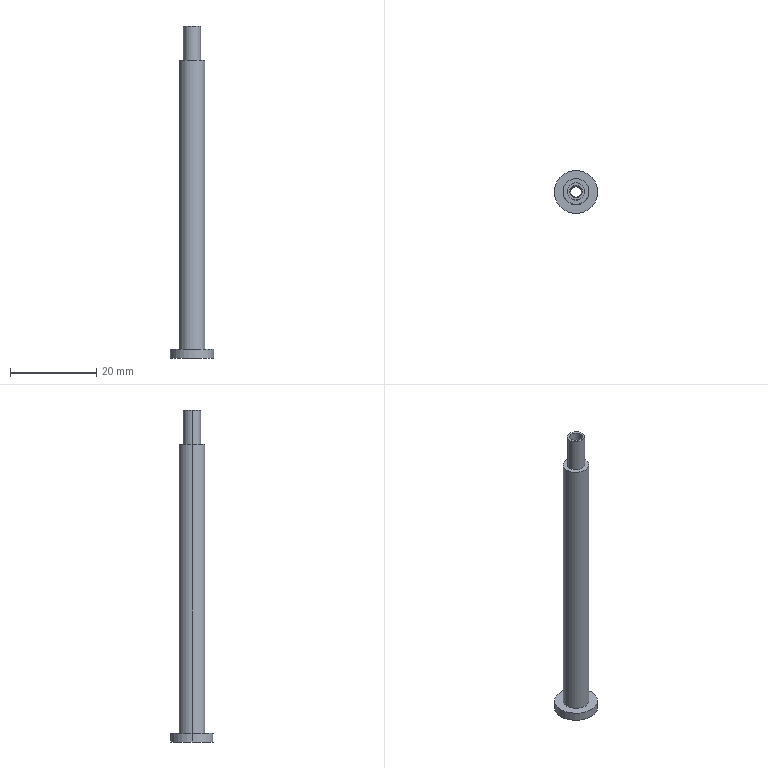Part | SolidWorks | features BaseBody 1 | 1 solid | 16 faces | box 10 x 10 x 77 mm | volume 1624 mm3 | cylinder 10 | plane 4 | cone 2 | commonest cylinder face diameters 2.459 x2 3 x2 4 x2 6 x2 10 x2
STEP:
#1=CARTESIAN_POINT('',(3.,0.,2.));
#2=VERTEX_POINT('',#1);
#3=CARTESIAN_POINT('',(-3.,0.,2.));
#4=VERTEX_POINT('',#3);
#5=CARTESIAN_POINT('',(0.,0.,2.));
#6=DIRECTION('',(0.,0.,1.));
#7=DIRECTION('',(1.,0.,0.));
#8=AXIS2_PLACEMENT_3D('',#5,#6,#7);
#9=CIRCLE('',#8,3.);
#10=EDGE_CURVE('',#2,#4,#9,.T.);
#11=ORIENTED_EDGE('',*,*,#10,.T.);
#12=CARTESIAN_POINT('',(-3.,0.,69.));
#13=VERTEX_POINT('',#12);
#14=CARTESIAN_POINT('',(-3.,0.,2.));
#15=DIRECTION('',(0.,0.,1.));
#16=VECTOR('',#15,1000.);
#17=LINE('',#14,#16);
#18=EDGE_CURVE('',#4,#13,#17,.T.);
#19=ORIENTED_EDGE('',*,*,#18,.T.);
#20=CARTESIAN_POINT('',(3.,0.,69.));
#21=VERTEX_POINT('',#20);
#22=CARTESIAN_POINT('',(0.,0.,69.));
#23=DIRECTION('',(0.,0.,-1.));
#24=DIRECTION('',(1.,0.,0.));
#25=AXIS2_PLACEMENT_3D('',#22,#23,#24);
#26=CIRCLE('',#25,3.);
#27=EDGE_CURVE('',#13,#21,#26,.T.);
#28=ORIENTED_EDGE('',*,*,#27,.T.);
#29=CARTESIAN_POINT('',(3.,0.,2.));
#30=DIRECTION('',(0.,0.,1.));
#31=VECTOR('',#30,1000.);
#32=LINE('',#29,#31);
#33=EDGE_CURVE('',#2,#21,#32,.T.);
#34=ORIENTED_EDGE('',*,*,#33,.F.);
#35=EDGE_LOOP('',(#11,#19,#28,#34));
#36=FACE_OUTER_BOUND('',#35,.T.);
#37=CARTESIAN_POINT('',(0.,0.,2.));
#38=DIRECTION('',(0.,0.,1.));
#39=DIRECTION('',(1.,0.,0.));
#40=AXIS2_PLACEMENT_3D('',#37,#38,#39);
#41=CYLINDRICAL_SURFACE('',#40,3.);
#42=ADVANCED_FACE('',(#36),#41,.T.);
#43=CARTESIAN_POINT('',(5.,0.,0.));
#44=VERTEX_POINT('',#43);
#45=CARTESIAN_POINT('',(-5.,0.,0.));
#46=VERTEX_POINT('',#45);
#47=CARTESIAN_POINT('',(0.,0.,0.));
#48=DIRECTION('',(0.,0.,1.));
#49=DIRECTION('',(1.,0.,0.));
#50=AXIS2_PLACEMENT_3D('',#47,#48,#49);
#51=CIRCLE('',#50,5.);
#52=EDGE_CURVE('',#44,#46,#51,.T.);
#53=ORIENTED_EDGE('',*,*,#52,.T.);
#54=CARTESIAN_POINT('',(-5.,0.,2.));
#55=VERTEX_POINT('',#54);
#56=CARTESIAN_POINT('',(-5.,0.,0.));
#57=DIRECTION('',(0.,0.,1.));
#58=VECTOR('',#57,1000.);
#59=LINE('',#56,#58);
#60=EDGE_CURVE('',#46,#55,#59,.T.);
#61=ORIENTED_EDGE('',*,*,#60,.T.);
#62=CARTESIAN_POINT('',(5.,0.,2.));
#63=VERTEX_POINT('',#62);
#64=CARTESIAN_POINT('',(0.,0.,2.));
#65=DIRECTION('',(0.,0.,-1.));
#66=DIRECTION('',(1.,0.,0.));
#67=AXIS2_PLACEMENT_3D('',#64,#65,#66);
#68=CIRCLE('',#67,5.);
#69=EDGE_CURVE('',#55,#63,#68,.T.);
#70=ORIENTED_EDGE('',*,*,#69,.T.);
#71=CARTESIAN_POINT('',(5.,0.,0.));
#72=DIRECTION('',(0.,0.,1.));
#73=VECTOR('',#72,1000.);
#74=LINE('',#71,#73);
#75=EDGE_CURVE('',#44,#63,#74,.T.);
#76=ORIENTED_EDGE('',*,*,#75,.F.);
#77=EDGE_LOOP('',(#53,#61,#70,#76));
#78=FACE_OUTER_BOUND('',#77,.T.);
#79=CARTESIAN_POINT('',(0.,0.,0.));
#80=DIRECTION('',(0.,0.,1.));
#81=DIRECTION('',(1.,0.,0.));
#82=AXIS2_PLACEMENT_3D('',#79,#80,#81);
#83=CYLINDRICAL_SURFACE('',#82,5.);
#84=ADVANCED_FACE('',(#78),#83,.T.);
#85=CARTESIAN_POINT('',(-2.,0.,77.));
#86=VERTEX_POINT('',#85);
#87=CARTESIAN_POINT('',(2.,0.,77.));
#88=VERTEX_POINT('',#87);
#89=CARTESIAN_POINT('',(0.,0.,77.));
#90=DIRECTION('',(0.,0.,-1.));
#91=DIRECTION('',(-1.,0.,0.));
#92=AXIS2_PLACEMENT_3D('',#89,#90,#91);
#93=CIRCLE('',#92,2.);
#94=EDGE_CURVE('',#86,#88,#93,.T.);
#95=ORIENTED_EDGE('',*,*,#94,.T.);
#96=CARTESIAN_POINT('',(2.,0.,69.));
#97=VERTEX_POINT('',#96);
#98=CARTESIAN_POINT('',(2.,0.,77.));
#99=DIRECTION('',(0.,0.,-1.));
#100=VECTOR('',#99,1000.);
#101=LINE('',#98,#100);
#102=EDGE_CURVE('',#88,#97,#101,.T.);
#103=ORIENTED_EDGE('',*,*,#102,.T.);
#104=CARTESIAN_POINT('',(-2.,0.,69.));
#105=VERTEX_POINT('',#104);
#106=CARTESIAN_POINT('',(0.,0.,69.));
#107=DIRECTION('',(0.,0.,1.));
#108=DIRECTION('',(-1.,0.,0.));
#109=AXIS2_PLACEMENT_3D('',#106,#107,#108);
#110=CIRCLE('',#109,2.);
#111=EDGE_CURVE('',#97,#105,#110,.T.);
#112=ORIENTED_EDGE('',*,*,#111,.T.);
#113=CARTESIAN_POINT('',(-2.,0.,77.));
#114=DIRECTION('',(0.,0.,-1.));
#115=VECTOR('',#114,1000.);
#116=LINE('',#113,#115);
#117=EDGE_CURVE('',#86,#105,#116,.T.);
#118=ORIENTED_EDGE('',*,*,#117,.F.);
#119=EDGE_LOOP('',(#95,#103,#112,#118));
#120=FACE_OUTER_BOUND('',#119,.T.);
#121=CARTESIAN_POINT('',(0.,0.,77.));
#122=DIRECTION('',(0.,0.,-1.));
#123=DIRECTION('',(-1.,0.,0.));
#124=AXIS2_PLACEMENT_3D('',#121,#122,#123);
#125=CYLINDRICAL_SURFACE('',#124,2.);
#126=ADVANCED_FACE('',(#120),#125,.T.);
#127=CARTESIAN_POINT('',(1.23,0.,6.837));
#128=VERTEX_POINT('',#127);
#129=CARTESIAN_POINT('',(0.,-1.23,6.837));
#130=VERTEX_POINT('',#129);
#131=CARTESIAN_POINT('',(0.,0.,6.837));
#132=DIRECTION('',(0.,0.,-1.));
#133=DIRECTION('',(-1.,0.,0.));
#134=AXIS2_PLACEMENT_3D('',#131,#132,#133);
#135=CIRCLE('',#134,1.23);
#136=EDGE_CURVE('',#128,#130,#135,.T.);
#137=ORIENTED_EDGE('',*,*,#136,.F.);
#138=CARTESIAN_POINT('',(1.23,0.,0.));
#139=VERTEX_POINT('',#138);
#140=CARTESIAN_POINT('',(1.23,0.,5.));
#141=DIRECTION('',(0.,0.,-1.));
#142=VECTOR('',#141,1000.);
#143=LINE('',#140,#142);
#144=EDGE_CURVE('',#128,#139,#143,.T.);
#145=ORIENTED_EDGE('',*,*,#144,.T.);
#146=CARTESIAN_POINT('',(-1.23,0.,0.));
#147=VERTEX_POINT('',#146);
#148=CARTESIAN_POINT('',(0.,0.,0.));
#149=DIRECTION('',(0.,0.,1.));
#150=DIRECTION('',(-1.,0.,0.));
#151=AXIS2_PLACEMENT_3D('',#148,#149,#150);
#152=CIRCLE('',#151,1.23);
#153=EDGE_CURVE('',#147,#139,#152,.T.);
#154=ORIENTED_EDGE('',*,*,#153,.F.);
#155=CARTESIAN_POINT('',(-1.23,0.,6.837));
#156=VERTEX_POINT('',#155);
#157=CARTESIAN_POINT('',(-1.23,0.,5.));
#158=DIRECTION('',(0.,0.,-1.));
#159=VECTOR('',#158,1000.);
#160=LINE('',#157,#159);
#161=EDGE_CURVE('',#156,#147,#160,.T.);
#162=ORIENTED_EDGE('',*,*,#161,.F.);
#163=CARTESIAN_POINT('',(0.,0.,6.837));
#164=DIRECTION('',(0.,0.,-1.));
#165=DIRECTION('',(-1.,0.,0.));
#166=AXIS2_PLACEMENT_3D('',#163,#164,#165);
#167=CIRCLE('',#166,1.23);
#168=EDGE_CURVE('',#130,#156,#167,.T.);
#169=ORIENTED_EDGE('',*,*,#168,.F.);
#170=EDGE_LOOP('',(#137,#145,#154,#162,#169));
#171=FACE_OUTER_BOUND('',#170,.T.);
#172=CARTESIAN_POINT('',(0.,0.,5.));
#173=DIRECTION('',(0.,0.,-1.));
#174=DIRECTION('',(-1.,0.,0.));
#175=AXIS2_PLACEMENT_3D('',#172,#173,#174);
#176=CYLINDRICAL_SURFACE('',#175,1.23);
#177=ADVANCED_FACE('',(#171),#176,.F.);
#178=CARTESIAN_POINT('',(-1.5,0.,7.));
#179=VERTEX_POINT('',#178);
#180=CARTESIAN_POINT('',(0.,-1.5,7.));
#181=VERTEX_POINT('',#180);
#182=CARTESIAN_POINT('',(0.,0.,7.));
#183=DIRECTION('',(0.,0.,1.));
#184=DIRECTION('',(1.,0.,0.));
#185=AXIS2_PLACEMENT_3D('',#182,#183,#184);
#186=CIRCLE('',#185,1.5);
#187=EDGE_CURVE('',#179,#181,#186,.T.);
#188=ORIENTED_EDGE('',*,*,#187,.F.);
#189=CARTESIAN_POINT('',(-1.5,0.,77.));
#190=VERTEX_POINT('',#189);
#191=CARTESIAN_POINT('',(-1.5,0.,42.));
#192=DIRECTION('',(0.,0.,1.));
#193=VECTOR('',#192,1000.);
#194=LINE('',#191,#193);
#195=EDGE_CURVE('',#179,#190,#194,.T.);
#196=ORIENTED_EDGE('',*,*,#195,.T.);
#197=CARTESIAN_POINT('',(1.5,0.,77.));
#198=VERTEX_POINT('',#197);
#199=CARTESIAN_POINT('',(0.,0.,77.));
#200=DIRECTION('',(0.,0.,1.));
#201=DIRECTION('',(1.,0.,0.));
#202=AXIS2_PLACEMENT_3D('',#199,#200,#201);
#203=CIRCLE('',#202,1.5);
#204=EDGE_CURVE('',#190,#198,#203,.T.);
#205=ORIENTED_EDGE('',*,*,#204,.T.);
#206=CARTESIAN_POINT('',(1.5,0.,7.));
#207=VERTEX_POINT('',#206);
#208=CARTESIAN_POINT('',(1.5,0.,42.));
#209=DIRECTION('',(0.,0.,1.));
#210=VECTOR('',#209,1000.);
#211=LINE('',#208,#210);
#212=EDGE_CURVE('',#207,#198,#211,.T.);
#213=ORIENTED_EDGE('',*,*,#212,.F.);
#214=CARTESIAN_POINT('',(0.,0.,7.));
#215=DIRECTION('',(0.,0.,1.));
#216=DIRECTION('',(1.,0.,0.));
#217=AXIS2_PLACEMENT_3D('',#214,#215,#216);
#218=CIRCLE('',#217,1.5);
#219=EDGE_CURVE('',#181,#207,#218,.T.);
#220=ORIENTED_EDGE('',*,*,#219,.F.);
#221=EDGE_LOOP('',(#188,#196,#205,#213,#220));
#222=FACE_OUTER_BOUND('',#221,.T.);
#223=CARTESIAN_POINT('',(0.,0.,42.));
#224=DIRECTION('',(0.,0.,1.));
#225=DIRECTION('',(1.,0.,0.));
#226=AXIS2_PLACEMENT_3D('',#223,#224,#225);
#227=CYLINDRICAL_SURFACE('',#226,1.5);
#228=ADVANCED_FACE('',(#222),#227,.F.);
#229=ORIENTED_EDGE('',*,*,#168,.T.);
#230=CARTESIAN_POINT('',(0.,1.23,6.837));
#231=VERTEX_POINT('',#230);
#232=CARTESIAN_POINT('',(0.,0.,6.837));
#233=DIRECTION('',(0.,0.,-1.));
#234=DIRECTION('',(-1.,0.,0.));
#235=AXIS2_PLACEMENT_3D('',#232,#233,#234);
#236=CIRCLE('',#235,1.23);
#237=EDGE_CURVE('',#156,#231,#236,.T.);
#238=ORIENTED_EDGE('',*,*,#237,.T.);
#239=CARTESIAN_POINT('',(0.,1.5,7.));
#240=VERTEX_POINT('',#239);
#241=CARTESIAN_POINT('',(0.,1.5,7.));
#242=DIRECTION('',(0.,0.8572,0.515));
#243=VECTOR('',#242,1000.);
#244=LINE('',#241,#243);
#245=EDGE_CURVE('',#231,#240,#244,.T.);
#246=ORIENTED_EDGE('',*,*,#245,.T.);
#247=CARTESIAN_POINT('',(0.,0.,7.));
#248=DIRECTION('',(0.,0.,1.));
#249=DIRECTION('',(1.,0.,0.));
#250=AXIS2_PLACEMENT_3D('',#247,#248,#249);
#251=CIRCLE('',#250,1.5);
#252=EDGE_CURVE('',#240,#179,#251,.T.);
#253=ORIENTED_EDGE('',*,*,#252,.T.);
#254=ORIENTED_EDGE('',*,*,#187,.T.);
#255=CARTESIAN_POINT('',(0.,-1.5,7.));
#256=DIRECTION('',(0.,-0.8572,0.515));
#257=VECTOR('',#256,1000.);
#258=LINE('',#255,#257);
#259=EDGE_CURVE('',#130,#181,#258,.T.);
#260=ORIENTED_EDGE('',*,*,#259,.F.);
#261=EDGE_LOOP('',(#229,#238,#246,#253,#254,#260));
#262=FACE_OUTER_BOUND('',#261,.T.);
#263=CARTESIAN_POINT('',(0.,0.,7.));
#264=DIRECTION('',(0.,0.,1.));
#265=DIRECTION('',(0.,-1.,0.));
#266=AXIS2_PLACEMENT_3D('',#263,#264,#265);
#267=CONICAL_SURFACE('',#266,1.5,1.03);
#268=ADVANCED_FACE('',(#262),#267,.F.);
#269=ORIENTED_EDGE('',*,*,#18,.F.);
#270=CARTESIAN_POINT('',(0.,0.,2.));
#271=DIRECTION('',(0.,0.,1.));
#272=DIRECTION('',(1.,0.,0.));
#273=AXIS2_PLACEMENT_3D('',#270,#271,#272);
#274=CIRCLE('',#273,3.);
#275=EDGE_CURVE('',#4,#2,#274,.T.);
#276=ORIENTED_EDGE('',*,*,#275,.T.);
#277=ORIENTED_EDGE('',*,*,#33,.T.);
#278=CARTESIAN_POINT('',(0.,0.,69.));
#279=DIRECTION('',(0.,0.,-1.));
#280=DIRECTION('',(1.,0.,0.));
#281=AXIS2_PLACEMENT_3D('',#278,#279,#280);
#282=CIRCLE('',#281,3.);
#283=EDGE_CURVE('',#21,#13,#282,.T.);
#284=ORIENTED_EDGE('',*,*,#283,.T.);
#285=EDGE_LOOP('',(#269,#276,#277,#284));
#286=FACE_OUTER_BOUND('',#285,.T.);
#287=CARTESIAN_POINT('',(0.,0.,2.));
#288=DIRECTION('',(0.,0.,1.));
#289=DIRECTION('',(1.,0.,0.));
#290=AXIS2_PLACEMENT_3D('',#287,#288,#289);
#291=CYLINDRICAL_SURFACE('',#290,3.);
#292=ADVANCED_FACE('',(#286),#291,.T.);
#293=ORIENTED_EDGE('',*,*,#10,.F.);
#294=ORIENTED_EDGE('',*,*,#275,.F.);
#295=EDGE_LOOP('',(#293,#294));
#296=FACE_BOUND('',#295,.T.);
#297=CARTESIAN_POINT('',(0.,0.,2.));
#298=DIRECTION('',(0.,0.,-1.));
#299=DIRECTION('',(1.,0.,0.));
#300=AXIS2_PLACEMENT_3D('',#297,#298,#299);
#301=CIRCLE('',#300,5.);
#302=EDGE_CURVE('',#63,#55,#301,.T.);
#303=ORIENTED_EDGE('',*,*,#302,.F.);
#304=ORIENTED_EDGE('',*,*,#69,.F.);
#305=EDGE_LOOP('',(#303,#304));
#306=FACE_OUTER_BOUND('',#305,.T.);
#307=CARTESIAN_POINT('',(0.,0.,2.));
#308=DIRECTION('',(0.,0.,-1.));
#309=DIRECTION('',(-1.,0.,0.));
#310=AXIS2_PLACEMENT_3D('',#307,#308,#309);
#311=PLANE('',#310);
#312=ADVANCED_FACE('',(#296,#306),#311,.F.);
#313=CARTESIAN_POINT('',(0.,0.,69.));
#314=DIRECTION('',(0.,0.,1.));
#315=DIRECTION('',(-1.,0.,0.));
#316=AXIS2_PLACEMENT_3D('',#313,#314,#315);
#317=CIRCLE('',#316,2.);
#318=EDGE_CURVE('',#105,#97,#317,.T.);
#319=ORIENTED_EDGE('',*,*,#318,.F.);
#320=ORIENTED_EDGE('',*,*,#111,.F.);
#321=EDGE_LOOP('',(#319,#320));
#322=FACE_BOUND('',#321,.T.);
#323=ORIENTED_EDGE('',*,*,#283,.F.);
#324=ORIENTED_EDGE('',*,*,#27,.F.);
#325=EDGE_LOOP('',(#323,#324));
#326=FACE_OUTER_BOUND('',#325,.T.);
#327=CARTESIAN_POINT('',(0.,0.,69.));
#328=DIRECTION('',(0.,0.,-1.));
#329=DIRECTION('',(-1.,0.,0.));
#330=AXIS2_PLACEMENT_3D('',#327,#328,#329);
#331=PLANE('',#330);
#332=ADVANCED_FACE('',(#322,#326),#331,.F.);
#333=ORIENTED_EDGE('',*,*,#60,.F.);
#334=CARTESIAN_POINT('',(0.,0.,0.));
#335=DIRECTION('',(0.,0.,1.));
#336=DIRECTION('',(1.,0.,0.));
#337=AXIS2_PLACEMENT_3D('',#334,#335,#336);
#338=CIRCLE('',#337,5.);
#339=EDGE_CURVE('',#46,#44,#338,.T.);
#340=ORIENTED_EDGE('',*,*,#339,.T.);
#341=ORIENTED_EDGE('',*,*,#75,.T.);
#342=ORIENTED_EDGE('',*,*,#302,.T.);
#343=EDGE_LOOP('',(#333,#340,#341,#342));
#344=FACE_OUTER_BOUND('',#343,.T.);
#345=CARTESIAN_POINT('',(0.,0.,0.));
#346=DIRECTION('',(0.,0.,1.));
#347=DIRECTION('',(1.,0.,0.));
#348=AXIS2_PLACEMENT_3D('',#345,#346,#347);
#349=CYLINDRICAL_SURFACE('',#348,5.);
#350=ADVANCED_FACE('',(#344),#349,.T.);
#351=ORIENTED_EDGE('',*,*,#102,.F.);
#352=CARTESIAN_POINT('',(0.,0.,77.));
#353=DIRECTION('',(0.,0.,-1.));
#354=DIRECTION('',(-1.,0.,0.));
#355=AXIS2_PLACEMENT_3D('',#352,#353,#354);
#356=CIRCLE('',#355,2.);
#357=EDGE_CURVE('',#88,#86,#356,.T.);
#358=ORIENTED_EDGE('',*,*,#357,.T.);
#359=ORIENTED_EDGE('',*,*,#117,.T.);
#360=ORIENTED_EDGE('',*,*,#318,.T.);
#361=EDGE_LOOP('',(#351,#358,#359,#360));
#362=FACE_OUTER_BOUND('',#361,.T.);
#363=CARTESIAN_POINT('',(0.,0.,77.));
#364=DIRECTION('',(0.,0.,-1.));
#365=DIRECTION('',(-1.,0.,0.));
#366=AXIS2_PLACEMENT_3D('',#363,#364,#365);
#367=CYLINDRICAL_SURFACE('',#366,2.);
#368=ADVANCED_FACE('',(#362),#367,.T.);
#369=ORIENTED_EDGE('',*,*,#153,.T.);
#370=CARTESIAN_POINT('',(0.,0.,0.));
#371=DIRECTION('',(0.,0.,1.));
#372=DIRECTION('',(-1.,0.,0.));
#373=AXIS2_PLACEMENT_3D('',#370,#371,#372);
#374=CIRCLE('',#373,1.23);
#375=EDGE_CURVE('',#139,#147,#374,.T.);
#376=ORIENTED_EDGE('',*,*,#375,.T.);
#377=EDGE_LOOP('',(#369,#376));
#378=FACE_BOUND('',#377,.T.);
#379=ORIENTED_EDGE('',*,*,#52,.F.);
#380=ORIENTED_EDGE('',*,*,#339,.F.);
#381=EDGE_LOOP('',(#379,#380));
#382=FACE_OUTER_BOUND('',#381,.T.);
#383=CARTESIAN_POINT('',(0.,0.,0.));
#384=DIRECTION('',(0.,0.,-1.));
#385=DIRECTION('',(-1.,0.,0.));
#386=AXIS2_PLACEMENT_3D('',#383,#384,#385);
#387=PLANE('',#386);
#388=ADVANCED_FACE('',(#378,#382),#387,.T.);
#389=CARTESIAN_POINT('',(0.,0.,77.));
#390=DIRECTION('',(0.,0.,1.));
#391=DIRECTION('',(1.,0.,0.));
#392=AXIS2_PLACEMENT_3D('',#389,#390,#391);
#393=CIRCLE('',#392,1.5);
#394=EDGE_CURVE('',#198,#190,#393,.T.);
#395=ORIENTED_EDGE('',*,*,#394,.F.);
#396=ORIENTED_EDGE('',*,*,#204,.F.);
#397=EDGE_LOOP('',(#395,#396));
#398=FACE_BOUND('',#397,.T.);
#399=ORIENTED_EDGE('',*,*,#94,.F.);
#400=ORIENTED_EDGE('',*,*,#357,.F.);
#401=EDGE_LOOP('',(#399,#400));
#402=FACE_OUTER_BOUND('',#401,.T.);
#403=CARTESIAN_POINT('',(0.,0.,77.));
#404=DIRECTION('',(0.,0.,-1.));
#405=DIRECTION('',(-1.,0.,0.));
#406=AXIS2_PLACEMENT_3D('',#403,#404,#405);
#407=PLANE('',#406);
#408=ADVANCED_FACE('',(#398,#402),#407,.F.);
#409=ORIENTED_EDGE('',*,*,#144,.F.);
#410=CARTESIAN_POINT('',(0.,0.,6.837));
#411=DIRECTION('',(0.,0.,-1.));
#412=DIRECTION('',(-1.,0.,0.));
#413=AXIS2_PLACEMENT_3D('',#410,#411,#412);
#414=CIRCLE('',#413,1.23);
#415=EDGE_CURVE('',#231,#128,#414,.T.);
#416=ORIENTED_EDGE('',*,*,#415,.F.);
#417=ORIENTED_EDGE('',*,*,#237,.F.);
#418=ORIENTED_EDGE('',*,*,#161,.T.);
#419=ORIENTED_EDGE('',*,*,#375,.F.);
#420=EDGE_LOOP('',(#409,#416,#417,#418,#419));
#421=FACE_OUTER_BOUND('',#420,.T.);
#422=CARTESIAN_POINT('',(0.,0.,5.));
#423=DIRECTION('',(0.,0.,-1.));
#424=DIRECTION('',(-1.,0.,0.));
#425=AXIS2_PLACEMENT_3D('',#422,#423,#424);
#426=CYLINDRICAL_SURFACE('',#425,1.23);
#427=ADVANCED_FACE('',(#421),#426,.F.);
#428=ORIENTED_EDGE('',*,*,#195,.F.);
#429=ORIENTED_EDGE('',*,*,#252,.F.);
#430=CARTESIAN_POINT('',(0.,0.,7.));
#431=DIRECTION('',(0.,0.,1.));
#432=DIRECTION('',(1.,0.,0.));
#433=AXIS2_PLACEMENT_3D('',#430,#431,#432);
#434=CIRCLE('',#433,1.5);
#435=EDGE_CURVE('',#207,#240,#434,.T.);
#436=ORIENTED_EDGE('',*,*,#435,.F.);
#437=ORIENTED_EDGE('',*,*,#212,.T.);
#438=ORIENTED_EDGE('',*,*,#394,.T.);
#439=EDGE_LOOP('',(#428,#429,#436,#437,#438));
#440=FACE_OUTER_BOUND('',#439,.T.);
#441=CARTESIAN_POINT('',(0.,0.,42.));
#442=DIRECTION('',(0.,0.,1.));
#443=DIRECTION('',(1.,0.,0.));
#444=AXIS2_PLACEMENT_3D('',#441,#442,#443);
#445=CYLINDRICAL_SURFACE('',#444,1.5);
#446=ADVANCED_FACE('',(#440),#445,.F.);
#447=ORIENTED_EDGE('',*,*,#245,.F.);
#448=ORIENTED_EDGE('',*,*,#415,.T.);
#449=ORIENTED_EDGE('',*,*,#136,.T.);
#450=ORIENTED_EDGE('',*,*,#259,.T.);
#451=ORIENTED_EDGE('',*,*,#219,.T.);
#452=ORIENTED_EDGE('',*,*,#435,.T.);
#453=EDGE_LOOP('',(#447,#448,#449,#450,#451,#452));
#454=FACE_OUTER_BOUND('',#453,.T.);
#455=CARTESIAN_POINT('',(0.,0.,7.));
#456=DIRECTION('',(0.,0.,1.));
#457=DIRECTION('',(0.,-1.,0.));
#458=AXIS2_PLACEMENT_3D('',#455,#456,#457);
#459=CONICAL_SURFACE('',#458,1.5,1.03);
#460=ADVANCED_FACE('',(#454),#459,.F.);
#461=CLOSED_SHELL('',(#42,#84,#126,#177,#228,#268,#292,#312,#332,#350,#368,#388,#408,#427,#446,#460));
#462=MANIFOLD_SOLID_BREP('',#461);
#463=CARTESIAN_POINT('',(0.,0.,0.));
#464=DIRECTION('',(0.,0.,1.));
#465=DIRECTION('',(1.,0.,0.));
#466=AXIS2_PLACEMENT_3D('',#463,#464,#465);
#467=(LENGTH_UNIT()NAMED_UNIT(*)SI_UNIT(.MILLI.,.METRE.));
#468=UNCERTAINTY_MEASURE_WITH_UNIT(LENGTH_MEASURE(0.00001),#467,'','');
#469=(NAMED_UNIT(*)PLANE_ANGLE_UNIT()SI_UNIT($,.RADIAN.));
#470=(NAMED_UNIT(*)SI_UNIT($,.STERADIAN.)SOLID_ANGLE_UNIT());
#471=(GEOMETRIC_REPRESENTATION_CONTEXT(3)GLOBAL_UNCERTAINTY_ASSIGNED_CONTEXT((#468))GLOBAL_UNIT_ASSIGNED_CONTEXT((#467,#469,#470))REPRESENTATION_CONTEXT('',''));
#472=ADVANCED_BREP_SHAPE_REPRESENTATION('',(#462,#466),#471);